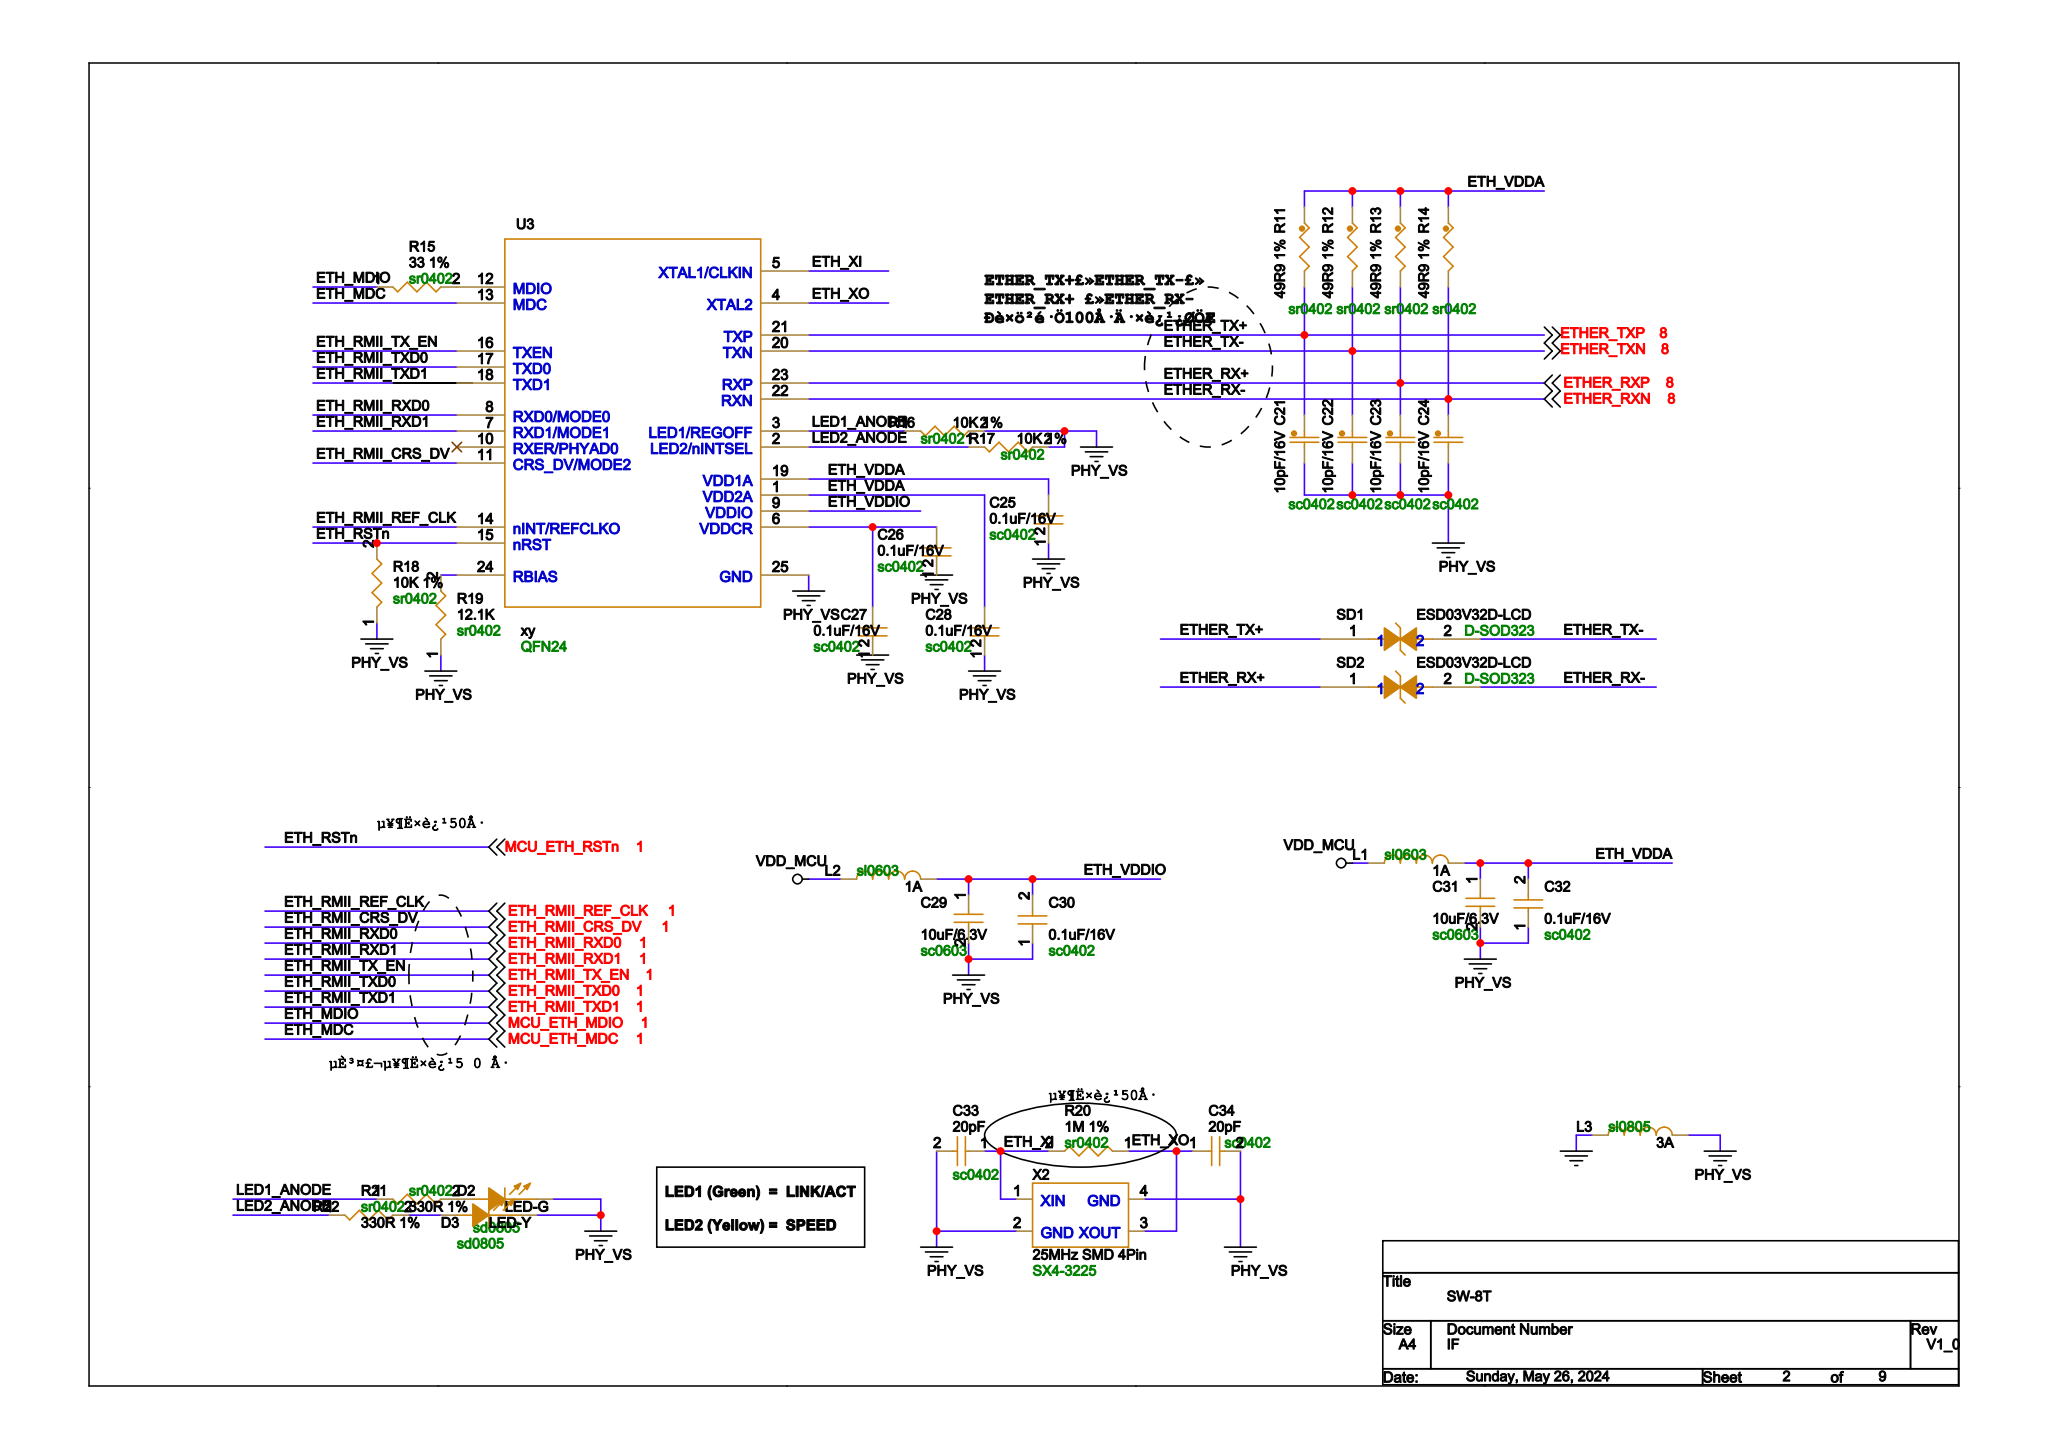Circuit board | Cadence Allegro | 399 parts | 387 nets | one sheet of the schematic
Parts on this sheet (reference | value | footprint):
C21 | 10pF/16V | SC0402
C25 | 0.1uF/16V | SC0402
C26 | 0.1uF/16V | SC0402
C27 | 0.1uF/16V | SC0402
C28 | 0.1uF/16V | SC0402
C29 | 10uF/6.3V | SC0603
C30 | 0.1uF/16V | SC0402
C31 | 10uF/6.3V | SC0603
C32 | 0.1uF/16V | SC0402
C33 | 20pF | SC0402
C34 | 20pF | SC0402
D2 | LED-G | SD0805
D3 | LED-Y | SD0805
L1 | 1A | SL0603
L2 | 1A | SL0603
L3 | 3A | SL0805
R11 | 49R9 1% | SR0402
R12 | 49R9 1% | SR0402
R13 | 49R9 1% | SR0402
R15 | 33 1% | SR0402
R16 | 10K 1% | SR0402
R17 | 10K 1% | SR0402
R18 | 10K 1% | SR0402
R19 | 12.1K | SR0402
R20 | 1M 1% | SR0402
R21 | 330R 1% | SR0402
R22 | 330R 1% | SR0402
SD1 | ESD03V32D-LCD | D-SOD323
SD2 | ESD03V32D-LCD | D-SOD323
U3 | xy | QFN24
X2 | 25MHz SMD 4Pin | SX4-3225
Nets of these parts (net: part-pin ...):
GND: L3-1
VDD_MCU: L1-1 L2-1
MCU_ETH_RSTN: R18-2 U3-15
ETHER_TXP: C21-1 R11-2 SD1-1 U3-21
PHY_VS: C21-2 C25-1 C26-1 C27-1 C28-1 C29-2 C30-1 C31-2 C32-1 C33-2 C34-2 D2-2 D3-2 L3-2 R16-2 R17-2 R18-1 R19-1 X2-2 X2-4 U3-25
ETHER_TXN: R12-2 SD1-2 U3-20
ETHER_RXP: R13-2 SD2-1 U3-23
ETHER_RXN: SD2-2 U3-22
ETH_VDDA: C25-2 C28-2 C31-1 C32-2 L1-2 R11-1 R12-1 R13-1 U3-1 U3-19
N17450796: C26-2 C27-2 U3-6
ETH_VDDIO: C29-1 C30-2 L2-2 U3-9
ETH_XI: C33-1 R20-2 X2-1 U3-5
ETH_XO: C34-1 R20-1 X2-3 U3-4
N174495431: D2-1 R21-2
N17468072: D3-1 R22-2
MCU_ETH_MDIO: R15-1
N1744727111: R15-2 U3-12
LED1_ANODE: R16-1 R21-1 U3-3
LED2_ANODE: R17-1 R22-1 U3-2
N17455797: R19-2 U3-24
ETH_RMII_REF_CLK: U3-14
ETH_RMII_CRS_DV: U3-11
ETH_RMII_TX_EN: U3-16
ETH_RMII_TXD0: U3-17
ETH_RMII_TXD1: U3-18
MCU_ETH_MDC: U3-13
ETH_RMII_RXD0: U3-8
ETH_RMII_RXD1: U3-7